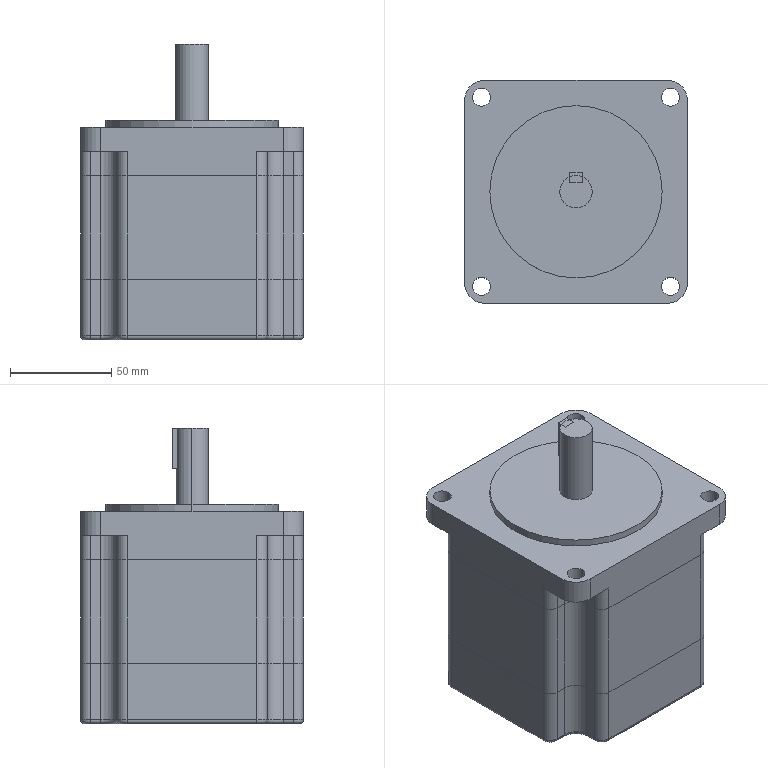Part | STEP file | bsbhb115-06 | 5 solids | 131 faces | box 110 x 110 x 146 mm | volume 1174749 mm3 | cylinder 64 | plane 55 | torus 12 | commonest cylinder face diameters 10 x24 16 x14 4 x12 8.865 x8 20 x4 85 x2